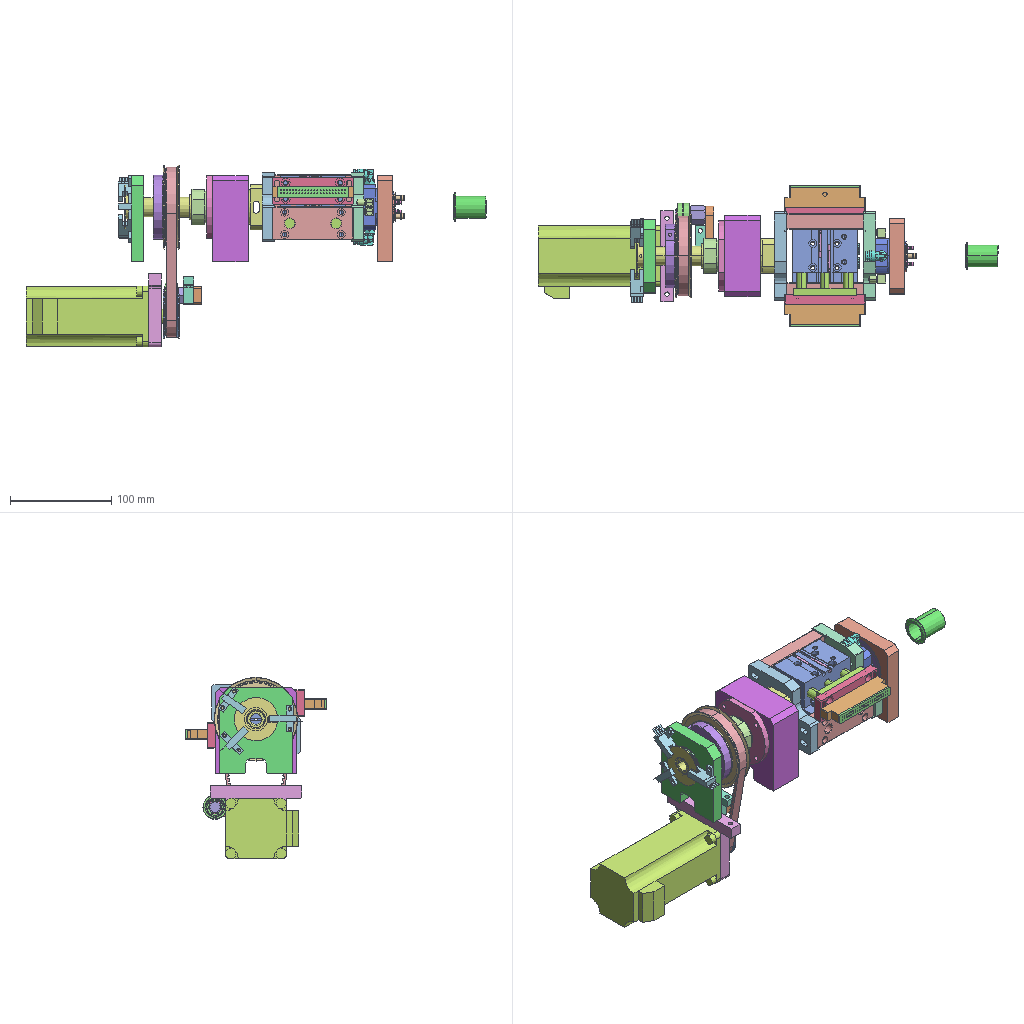Assembly | SolidWorks | 45 different items | 69 placed | box 454 x 139 x 179 mm
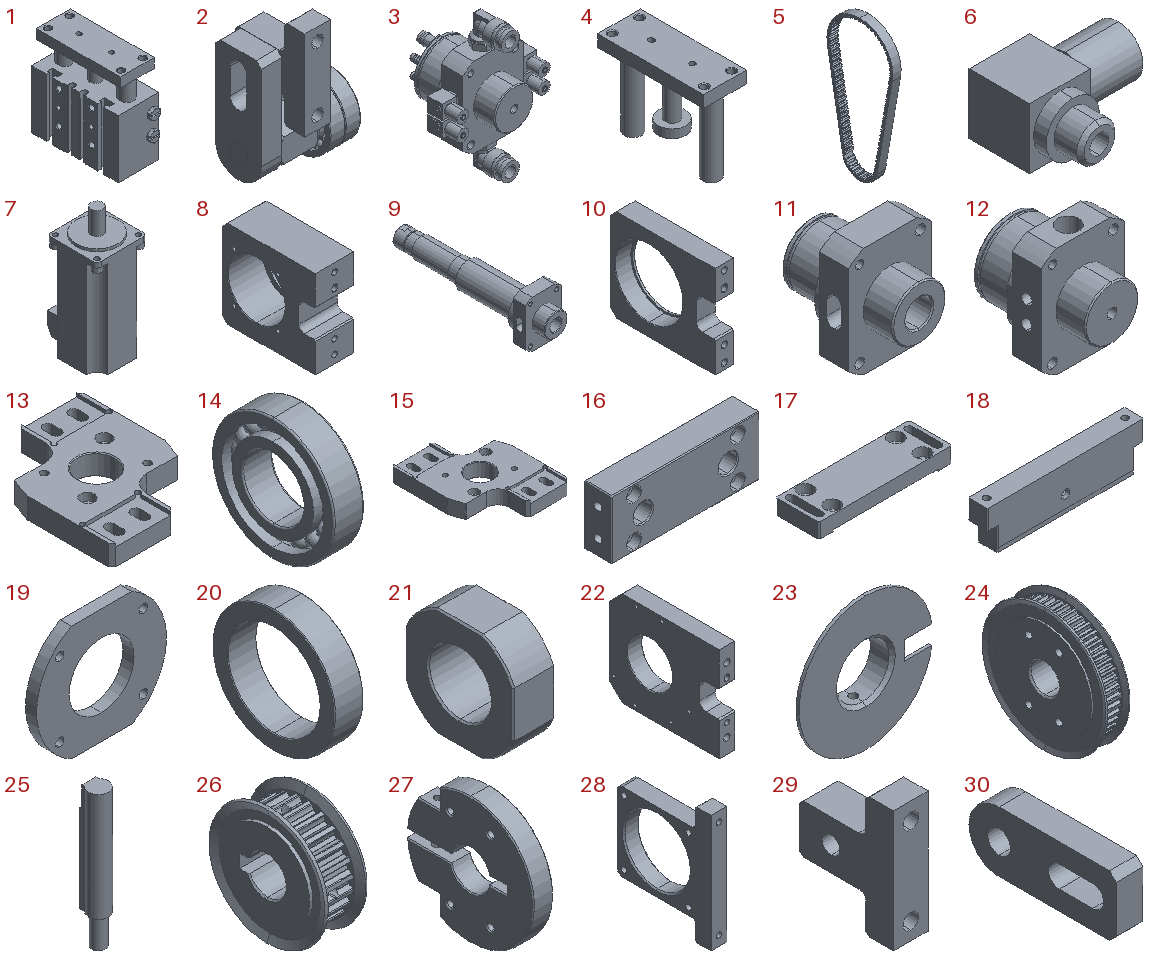Parts list (item | name | quantity | parent item | size | volume | features):
1 | (subassembly) | x2 | - | 30 x 66.5 x 66 mm | 82906 mm3 | -
2 | (subassembly) | x1 | - | 38 x 30 x 57.5 mm | 18168 mm3 | features AEMSimFeature 1
3 | (subassembly) | x1 | - | 54 x 52.5 x 75 mm | 38133 mm3 | -
4 | - | x2 | in 1 | 25 x 62 x 51.5 mm | 19698 mm3 | features ICE 4, RevCut 4, RefAxis 3, HoleWzd 2, 3DProfileFeature 1, Extrusion 1, Revolution 1
5 | - | x1 | - | 10 x 78.83 x 168.305 mm | 10817 mm3 | features CurvePattern 1, ExtruThin 1, ICE 1
6 | - | x4 | in 3 | 16.5 x 13.5 x 8 mm | 829.104 mm3 | features BaseBody 1, MoveCopyBody 1
7 | - | x1 | - | 60 x 72 x 151.5 mm | 401427 mm3 | features ICE 5, Chamfer 1, Extrusion 1, Fillet 1, HoleWzd 1
8 | - | x1 | - | 35 x 85 x 80 mm | 150248 mm3 | features Chamfer 3, HoleWzd 2, Cut 1, Extrusion 1, Fillet 1, ICE 1
9 | - | x1 | - | 34 x 148 x 45 mm | 55007 mm3 | features ICE 6, Chamfer 2, HoleWzd 1, Revolution 1
10 | - | x1 | - | 15 x 85 x 75 mm | 53244 mm3 | features Chamfer 3, ICE 2, Extrusion 1, HoleWzd 1
11 | - | x1 | - | 34 x 44 x 45 mm | 26629 mm3 | features ICE 4, Chamfer 2, HoleWzd 1, Revolution 1
12 | - | x1 | in 3 | 34 x 42 x 45 mm | 29276 mm3 | features ICE 10, HoleWzd 7, Chamfer 2, Revolution 1
13 | - | x1 | - | 68 x 87 x 12 mm | 40763 mm3 | features Chamfer 3, Cut 2, Fillet 2, ICE 2, Extrusion 1, HoleWzd 1
14 | - | x2 | in 2 | 6 x 24 x 24 mm | 1508 mm3 | features Stock 1
15 | - | x1 | - | 68 x 87 x 12 mm | 40763 mm3 | features Chamfer 3, Fillet 2, ICE 2, Cut 1, Extrusion 1, HoleWzd 1
16 | - | x2 | - | 80 x 15 x 32 mm | 33801 mm3 | features HoleWzd 3, Chamfer 1, Cut 1, ExtruThin 1
17 | - | x2 | - | 80 x 26 x 9 mm | 13853 mm3 | features ICE 4, Chamfer 1, Extrusion 1, MirrorPattern 1
18 | - | x2 | - | 80 x 10 x 22 mm | 14660 mm3 | features ICE 6, Chamfer 2, HoleWzd 2, Extrusion 1, LPattern 1
19 | - | x1 | - | 70 x 8 x 62 mm | 17164 mm3 | features HoleWzd 1, ICE 1, Revolution 1
20 | - | x1 | - | 8 x 34 x 34 mm | 3170 mm3 | features Chamfer 1, Extrusion 1
21 | - | x1 | - | 15 x 35 x 35 mm | 10821 mm3 | features ICE 2, Chamfer 1, Extrusion 1
22 | - | x1 | - | 12 x 85 x 73 mm | 56726 mm3 | features Chamfer 3, HoleWzd 2, Extrusion 1, ICE 1
23 | - | x1 | - | 42.79 x 7 x 43 mm | 2222 mm3 | features Chamfer 2, CirPattern 1, HoleWzd 1, ICE 1, Revolution 1
24 | - | x1 | - | 16 x 82.872 x 82.872 mm | 61065 mm3 | features ICE 2, Chamfer 1, HoleWzd 1, RevCut 1, Revolution 1
25 | - | x4 | in 1 | 4 x 4.5 x 28 mm | 345.122 mm3 | features ICE 3, RefAxis 3, 3DProfileFeature 1, Extrusion 1
26 | - | x1 | - | 16 x 43.859 x 43.859 mm | 13285 mm3 | features ICE 3, HoleWzd 2, Chamfer 1, RevCut 1, Revolution 1
27 | - | x1 | - | 10 x 62.936 x 63 mm | 24833 mm3 | features HoleWzd 3, Chamfer 1, Extrusion 1
28 | - | x1 | - | 12 x 72 x 90 mm | 31178 mm3 | features Chamfer 2, Fillet 2, HoleWzd 2, Extrusion 1
29 | - | x1 | in 2 | 10 x 27 x 35 mm | 4690 mm3 | features HoleWzd 2, Chamfer 1, Extrusion 1, Fillet 1
30 | - | x1 | in 2 | 8 x 44 x 18 mm | 4950 mm3 | features Chamfer 1, Extrusion 1, HoleWzd 1
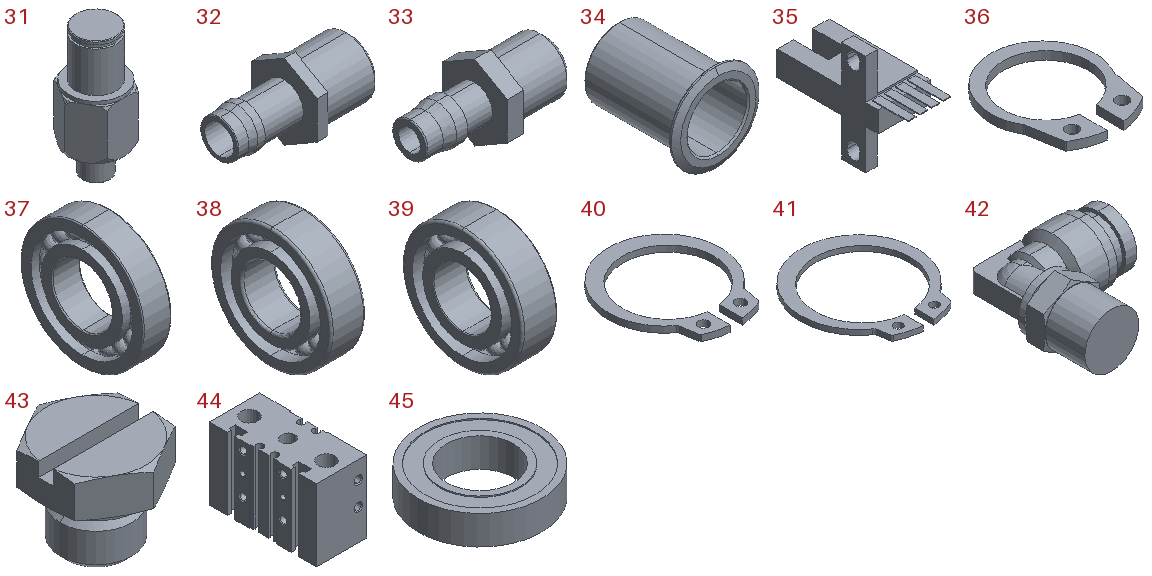31 | - | x1 | in 2 | 18.475 x 16 x 38 mm | 5453 mm3 | features Cut 3, ICE 3, Chamfer 1, Extrusion 1, RevCut 1
32 | - | x2 | in 3 | 18 x 9 x 10.392 mm | 450.495 mm3 | features Chamfer 1, Fillet 1, ICE 1, Revolution 1
33 | - | x4 | in 3 | 12.5 x 6 x 6.928 mm | 156.103 mm3 | features Chamfer 1, Fillet 1, ICE 1, Revolution 1
34 | - | x1 | - | 28 x 32 x 28 mm | 3444 mm3 | features Chamfer 2, Revolution 1
35 | - | x3 | - | 13.4 x 32.558 x 26 mm | 2213 mm3 | features ICE 6, Extrusion 1, LPattern 1
36 | - | x1 | in 2 | 12.5 x 14.97 x 1 mm | 58.29 mm3 | features MoveCopyBody 1, Stock 1
37 | - | x1 | - | 8 x 35 x 35 mm | 4447 mm3 | features MoveCopyBody 1, Stock 1
38 | - | x1 | - | 15 x 52 x 52 mm | 17866 mm3 | features Stock 1
39 | - | x2 | - | 15 x 52 x 52 mm | 17216 mm3 | features Stock 1
40 | - | x1 | - | 18.2 x 20.685 x 1 mm | 104.691 mm3 | features MoveCopyBody 1, Stock 1
41 | - | x1 | - | 27.2 x 29.88 x 1.2 mm | 261.105 mm3 | features MoveCopyBody 1, Stock 1
42 | - | x2 | in 3 | 20.9 x 22.1 x 11.547 mm | 2008 mm3 | features ICE 2, Revolution 2, HoleWzd 1
43 | - | x4 | in 1 | 7 x 8.083 x 6.5 mm | 175.846 mm3 | features RefAxis 3, ICE 2, 3DProfileFeature 1, Revolution 1
44 | - | x2 | in 1 | 30 x 64 x 43 mm | 62167 mm3 | features RefAxis 15, HoleWzd 11, 3DProfileFeature 5, RevCut 5, ICE 2, Extrusion 1, LPattern 1
45 | - | x1 | - | 55 x 55 x 13 mm | 20829 mm3 | features Extrusion 1, ICE 1, MirrorPattern 1
Mates (type | each side: item.copy, entity, surface, feature):
In the top assembly
Coincident | 16.1 face plane Extrude-Thin1 | 44.1 face plane Boss-Extrude1
Coincident | 16.1 face plane Extrude-Thin1 | 16.2 face plane Extrude-Thin1
Coincident | 16.2 face plane Extrude-Thin1 | 44.2 face plane Boss-Extrude1
Concentric | 17.1 face cylinder Cut-Extrude1 | 4.1 face cylinder Cut-Revolve3
Concentric | 17.1 face cylinder Cut-Extrude2 | 4.1 face cylinder Cut-Revolve2
Coincident | 4.1 face plane Boss-Extrude1 | 17.1 face plane Cut-Extrude5
Width | 17.1 face plane Cut-Extrude3 | 17.1 face plane Cut-Extrude3 | 18.1 face
Width | 17.1 face plane Mirror1 | 17.1 face plane Mirror1 | 18.1 face cylinder M4 Tapped Hole1
Coincident | 18.1 face plane Boss-Extrude1 | 17.1 face plane Boss-Extrude1
LimitDistanceDim | 18.1 face plane Boss-Extrude1 | 17.1 face plane Boss-Extrude1
Concentric | 17.2 face cylinder Cut-Extrude1 | 4.2 face cylinder Cut-Revolve3
Concentric | 17.2 face cylinder Cut-Extrude1 | 4.2 face cylinder Cut-Revolve2
Coincident | 4.2 face plane Boss-Extrude1 | 17.2 face plane Cut-Extrude5
Coincident | 17.2 face plane Boss-Extrude1 | 18.2 face plane Boss-Extrude1
Width | 17.2 face plane Cut-Extrude3 | 17.2 face plane Cut-Extrude3 | 18.2 face cylinder M4 Tapped Hole1
Width | 17.2 face plane Mirror1 | 17.2 face plane Mirror1 | 18.2 face cylinder M4 Tapped Hole1
LimitDistanceDim | 18.2 face plane Boss-Extrude1 | 17.2 face plane Boss-Extrude1
Concentric | 16.1 face cylinder Hole size by socket head cap screw type1 | 44.1 face cylinder LPattern1 | 2 times
Concentric | 16.2 face cylinder Hole size by socket head cap screw type1 | 44.2 face cylinder LPattern1 | 2 times
Coincident | 8.1 face plane Boss-Extrude1 | 10.1 face plane Boss-Extrude2
Concentric | 9.1 face cylinder Revolve1 | 20.1 face cylinder Boss-Extrude1
Concentric | 9.1 face cylinder Revolve1 | 21.1 face cylinder Boss-Extrude1
Coincident | 20.1 face plane Boss-Extrude1 | 21.1 face plane Boss-Extrude1
Coincident | 15.1 face plane Boss-Extrude1 | 9.1 face plane Revolve1
Width | 16.2 face plane Extrude-Thin1 | 16.2 face plane Extrude-Thin1 | 15.1 face plane Cut-Extrude2 | 15.1 face plane Boss-Extrude1
Coincident | 16.2 face plane Extrude-Thin1 | 15.1 face plane Cut-Extrude3
Width | 15.1 face plane Cut-Extrude2 | 15.1 face plane Boss-Extrude1 | 16.1 face plane Extrude-Thin1 | 16.1 face plane Extrude-Thin1
Width | 13.1 face plane Boss-Extrude1 | 13.1 face plane Cut-Extrude2 | 16.2 face plane Extrude-Thin1 | 16.2 face plane Extrude-Thin1
Coincident | 16.1 face plane Extrude-Thin1 | 13.1 face plane Cut-Extrude5
Concentric | 15.1 face cylinder Hole size by socket head cap screw type0 | 9.1 face cylinder M4 Tapped Hole2 | 2 times
Concentric | 13.1 face cylinder Cut-Extrude4 | 11.1 face cylinder Cut-Extrude5
Coincident | 13.1 face plane Boss-Extrude1 | 11.1 face plane Revolve1
Concentric | 9.1 face cylinder Revolve1 | 39.1 face cylinder Rolling bearings S7205 GB 292-94
Concentric | 9.1 face cylinder Revolve1 | 39.2 face cylinder Rolling bearings S7205 GB 292-94
Coincident | 39.2 face plane Rolling bearings S7205 GB 292-94 | 9.1 face plane Revolve1
Coincident | 39.1 face plane Rolling bearings S7205 GB 292-94 | 39.2 face plane Rolling bearings S7205 GB 292-94
Coincident | 39.2 face plane Rolling bearings S7205 GB 292-94 | 8.1 face plane Cut-Extrude2
Concentric | 8.1 face cylinder Cut-Extrude2 | 39.1 face cylinder Rolling bearings S7205 GB 292-94
Concentric | 8.1 face cylinder M4 Tapped Hole1 | 19.1 face cylinder Ø4.5 (4.5) Diameter Hole1 | 2 times
Coincident | 19.1 face plane Revolve1 | 39.1 face plane Rolling bearings S7205 GB 292-94
Coincident | 20.1 face plane Boss-Extrude1 | 39.1 face plane Rolling bearings S7205 GB 292-94
Concentric | 11.1 face cylinder Revolve1 | 38.1 face cylinder Rolling bearings 6205 GB 276-94
Coincident | 11.1 face plane Revolve1 | 38.1 face plane Rolling bearings 6205 GB 276-94
Concentric | 10.1 face cylinder Boss-Extrude2 | 38.1 face cylinder Rolling bearings 6205 GB 276-94
Coincident | 10.1 face plane Boss-Extrude2 | 38.1 face plane Rolling bearings 6205 GB 276-94
Concentric | 9.1 face cylinder Revolve1 | 24.1 face cylinder Cut-Extrude2
Coincident | 9.1 face plane Revolve1 | 24.1 face plane Revolve1
Concentric | 24.1 face cylinder Hole size by socket head cap screw type1 | 27.1 face cylinder M4 Tapped Hole2 | 2 times
Coincident | 24.1 face plane Revolve1 | 27.1 face plane Boss-Extrude1
Parallel | 8.1 face plane Boss-Extrude1 | 22.1 face plane Boss-Extrude1
DistanceDim | 8.1 face plane Boss-Extrude1 | 28.1 face plane Boss-Extrude1
Coincident | 8.1 plane | 28.1 plane
Concentric | 7.1 face cylinder Ø5.5 (5.5) Diameter Hole1 | 28.1 face cylinder M5 Tapped Hole1 | 2 times
Coincident | 7.1 face plane Boss-Extrude3 | 28.1 face plane Boss-Extrude1
Concentric | 26.1 face cylinder Cut-Extrude2 | 7.1 face cylinder Boss-Extrude1
Coincident | 26.1 face plane Revolve1 | 7.1 face plane Boss-Extrude1
Coincident | 24.1 face plane Cut-Extrude1 | 26.1 face plane Cut-Extrude1
Concentric | 24.1 face cylinder Revolve1 | 5.1 face cylinder Extrude-Thin1
DistanceDim | 5.1 face plane Extrude-Thin1 | 24.1 face plane Cut-Extrude1
Coincident | 24.1 plane | 26.1 plane
Coincident | 5.1 plane | 26.1 plane
DistanceDim | 28.1 face plane Boss-Extrude1 | 29.1 face plane Boss-Extrude1
DistanceDim | 14.1 face plane Rolling bearings 61901 GB 276-94 | 5.1 face plane Extrude-Thin1
DistanceDim | 29.1 face plane Boss-Extrude1 | 28.1 face plane Boss-Extrude1
Parallel | 9.1 face plane Cut-Extrude8 | 22.1 face plane Boss-Extrude1
Width | 35.1 face plane Cut-Extrude2 | 35.1 face plane Cut-Extrude2 | 22.1 face cylinder M3 Tapped Hole1 | 2 times
Coincident | 22.1 face plane Boss-Extrude1 | 35.1 face plane Boss-Extrude1
Concentric | 9.1 face cylinder Revolve1 | 23.1 face cylinder Revolve1
Coincident | 9.1 face plane Revolve1 | 23.1 face plane Revolve1
Width | 13.1 face plane Cut-Extrude2 | 13.1 face plane Boss-Extrude1 | 16.1 face plane Extrude-Thin1 | 16.1 face plane Extrude-Thin1
DistanceDim | 15.1 face plane Boss-Extrude1 | 16.1 face plane Extrude-Thin1
DistanceDim | 16.2 face plane Extrude-Thin1 | 15.1 face plane Boss-Extrude1
Concentric | 9.1 face cylinder Revolve1 | 40.1 face cylinder GB_CONNECTING_PIECE_RING_RRA 16
Coincident | 9.1 face plane Revolve1 | 40.1 face plane GB_CONNECTING_PIECE_RING_RRA 16
Concentric | 9.1 face cylinder Revolve1 | 37.1 face cylinder 6003ZZ
Coincident | 9.1 face plane Revolve1 | 37.1 face plane 6003ZZ
Concentric | 11.1 face cylinder Revolve1 | 41.1 face cylinder GB_CONNECTING_PIECE_RING_RRA 24
Coincident | 11.1 face plane Revolve1 | 41.1 face plane GB_CONNECTING_PIECE_RING_RRA 24
Coincident | 22.1 face plane Boss-Extrude1 | 35.2 face plane Boss-Extrude1
Coincident | 22.1 face plane Boss-Extrude1 | 35.3 face plane Boss-Extrude1
Concentric | 22.1 face cylinder M3 Tapped Hole1 | 35.2 face cylinder Cut-Extrude2 | 2 times
Concentric | 22.1 face cylinder M3 Tapped Hole1 | 35.3 face cylinder Cut-Extrude2 | 2 times
Concentric | 13.1 face cylinder Cut-Extrude4 | 12.1 face cylinder Cut-Extrude5 | 2 times
Coincident | 13.1 face plane Boss-Extrude1 | 12.1 face plane Revolve1
Concentric | 10.1 face cylinder Boss-Extrude2 | 45.1 face cylinder Boss-Extrude1
Coincident | 12.1 face plane Revolve1 | 45.1 face plane Boss-Extrude1
Concentric | 12.1 face cylinder Revolve1 | 34.1 face cylinder Revolve1
DistanceDim | 10.1 face plane Boss-Extrude2 | 34.1 face plane Revolve1
In subassembly 3
Concentric | 12.2 face cylinder M5 Tapped Hole1 | 6.1 face cylinder Input1
Concentric | 12.2 face cylinder M5 Tapped Hole1 | 6.2 face cylinder Input1
Coincident | 12.2 face plane Cut-Extrude1 | 6.2 face plane Input1
Coincident | 12.2 face plane Cut-Extrude1 | 6.1 face plane Input1
Parallel | 6.2 face plane Input1 | 6.1 face plane Input1
Parallel | 6.2 face plane Input1 | 12.2 face plane Cut-Extrude1
Concentric | 12.2 face cylinder M5 Tapped Hole3 | 6.3 face cylinder Input1
Concentric | 12.2 face cylinder M5 Tapped Hole3 | 6.4 face cylinder Input1
Coincident | 12.2 face plane Cut-Extrude1 | 6.3 face plane Input1
Coincident | 12.2 face plane Cut-Extrude1 | 6.4 face plane Input1
Parallel | 12.2 face plane Cut-Extrude1 | 6.3 face plane Input1
Parallel | 12.2 face plane Cut-Extrude1 | 6.4 face plane Input1
Coincident | 12.2 face plane Revolve1 | 33.1 face plane Revolve1
Coincident | 12.2 face plane Revolve1 | 33.2 face plane Revolve1
Coincident | 12.2 face plane Revolve1 | 33.3 face plane Revolve1
Coincident | 12.2 face plane Revolve1 | 33.4 face plane Revolve1
Concentric | 12.2 face cylinder M5 Tapped Hole2 | 33.1 face cylinder Revolve1
Concentric | 12.2 face cylinder M5 Tapped Hole2 | 33.2 face cylinder Revolve1
Concentric | 12.2 face cylinder M5 Tapped Hole2 | 33.3 face cylinder Revolve1
Concentric | 12.2 face cylinder M5 Tapped Hole2 | 33.4 face cylinder Revolve1
Concentric | 12.2 face cylinder G1/8 Tapped Hole1 | 42.1 face cylinder Revolve1
Coincident | 12.2 face plane Cut-Extrude1 | 42.1 face plane Revolve1
Concentric | 12.2 face cylinder G1/8 Tapped Hole2 | 42.2 face cylinder Revolve1
Coincident | 12.2 face plane Cut-Extrude1 | 42.2 face plane Revolve1
Parallel | 12.2 face plane Cut-Extrude1 | 42.2 face plane Boss-Extrude1
Parallel | 12.2 face plane Cut-Extrude1 | 42.1 face plane Boss-Extrude1
Concentric | 12.2 face cylinder M8 Tapped Hole1 | 32.1 face cylinder Revolve1
Coincident | 12.2 face plane Revolve1 | 32.1 face plane Revolve1
Concentric | 12.2 face cylinder M8 Tapped Hole1 | 32.2 face cylinder Revolve1
Coincident | 12.2 face plane Revolve1 | 32.2 face plane Revolve1
In subassembly 2
Concentric | 29.2 face cylinder M6 Tapped Hole1 | 30.1 face cylinder Boss-Extrude1
Concentric | 30.1 face cylinder M8 Tapped Hole1 | 31.1 face cylinder Boss-Extrude2
Coincident | 30.1 face plane Boss-Extrude1 | 31.1 face plane Boss-Extrude1
Concentric | 31.1 face cylinder Cut-Extrude4 | 14.2 face cylinder Rolling bearings 61901 GB 276-94
Coincident | 31.1 face plane Cut-Extrude4 | 14.2 face plane Rolling bearings 61901 GB 276-94
Concentric | 31.1 face cylinder Cut-Extrude4 | 14.3 face cylinder Rolling bearings 61901 GB 276-94
Coincident | 14.2 face plane Rolling bearings 61901 GB 276-94 | 14.3 face plane Rolling bearings 61901 GB 276-94
Coincident | 29.2 face plane Boss-Extrude1 | 30.1 face plane Boss-Extrude1 | 2 times
Concentric | 31.1 face cylinder Cut-Extrude5 | 36.1 face cylinder GB_CONNECTING_PIECE_RING_RRA 11
Coincident | 31.1 face plane Cut-Extrude5 | 36.1 face plane GB_CONNECTING_PIECE_RING_RRA 11
In subassembly 1
Concentric | 44.3 face cylinder Hole7 | 4.3 face cylinder Boss-Extrude2
Concentric | 44.3 face cylinder Hole8 | 4.3 face cylinder Boss-Extrude3
LimitDistanceDim | 4.3 face plane Revolve1 | 44.3 face plane Cut-Revolve1
Coincident | 44.3 face plane Boss-Extrude1 | 43.1 face plane Revolve1
Coincident | 44.3 face plane Boss-Extrude1 | 43.2 face plane Revolve1
Concentric | 44.3 face cylinder Hole3 | 43.2 face cylinder Revolve1
Tangent | 43.1 face cylinder Revolve1 | 44.3 face cylinder Hole4
Concentric | 44.3 face cylinder Boss-Extrude1 | 25.1 face cylinder Boss-Extrude1
Parallel | 44.3 face plane Boss-Extrude1 | 25.1 face plane Boss-Extrude2
Coincident | 44.3 face plane Boss-Extrude1 | 25.1 face plane Boss-Extrude1
Concentric | 44.3 face cylinder Boss-Extrude1 | 25.2 face cylinder Boss-Extrude1
Parallel | 44.3 face plane Boss-Extrude1 | 25.2 face plane Boss-Extrude2
Coincident | 44.3 face plane Boss-Extrude1 | 25.2 face plane Boss-Extrude1